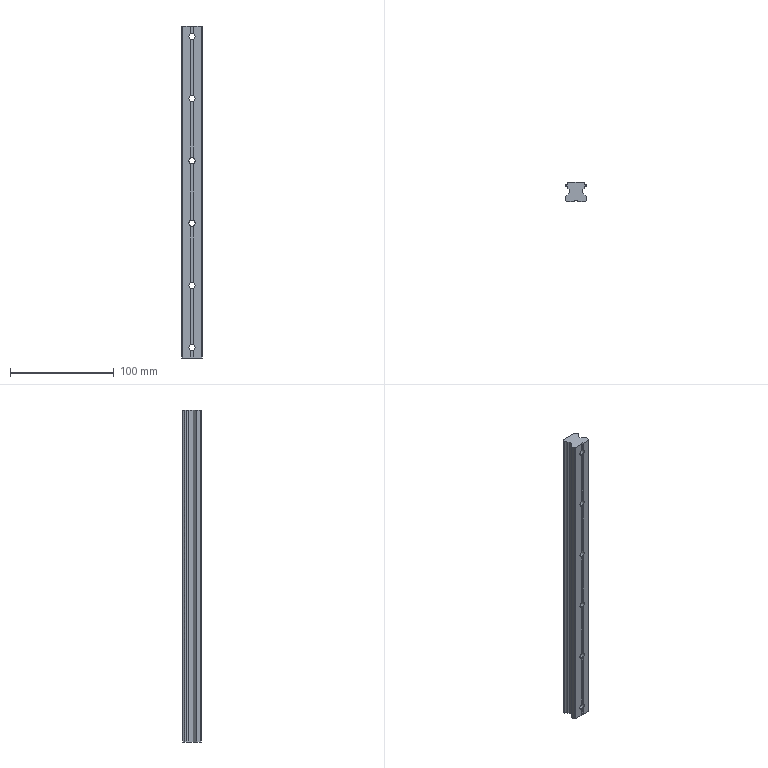Part | SolidWorks | features ICE 9, Chamfer 3, Fillet 3, HoleWzd 2, Extrusion 1 | 1 solid | 165 faces | box 20 x 18 x 320 mm | volume 90311 mm3 | plane 88 | cylinder 53 | cone 24 | commonest cylinder face diameters 6 x12 9.5 x12 0.156 x8 4.475 x4 0.617 x2 0.984 x2